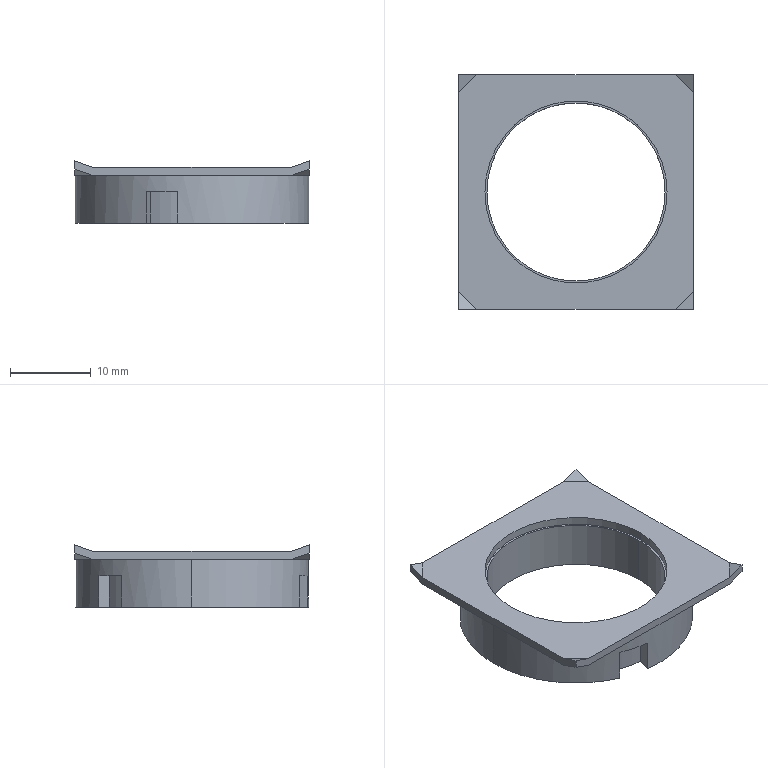Part | STEP file | A22NE_M_N_NUT | 1 solid | 34 faces | box 29 x 29 x 7.7 mm | volume 1960 mm3 | plane 25 | cylinder 9 | commonest cylinder face diameters 25.2 x3 22 x2 22.5 x2 28.8 x2
STEP:
#1=CARTESIAN_POINT('',(-11.25,0.,-0.8));
#2=VERTEX_POINT('',#1);
#3=CARTESIAN_POINT('',(11.25,0.,-0.8));
#4=VERTEX_POINT('',#3);
#5=CARTESIAN_POINT('',(0.,0.,-0.8));
#6=DIRECTION('',(0.,0.,1.));
#7=DIRECTION('',(1.,0.,0.));
#8=AXIS2_PLACEMENT_3D('',#5,#6,#7);
#9=CIRCLE('',#8,11.25);
#10=EDGE_CURVE('',#2,#4,#9,.T.);
#11=ORIENTED_EDGE('',*,*,#10,.T.);
#12=CARTESIAN_POINT('',(11.25,0.,-1.8));
#13=VERTEX_POINT('',#12);
#14=CARTESIAN_POINT('',(11.25,0.,-0.8));
#15=DIRECTION('',(0.,0.,-1.));
#16=VECTOR('',#15,1000.);
#17=LINE('',#14,#16);
#18=EDGE_CURVE('',#4,#13,#17,.T.);
#19=ORIENTED_EDGE('',*,*,#18,.T.);
#20=CARTESIAN_POINT('',(-11.25,0.,-1.8));
#21=VERTEX_POINT('',#20);
#22=CARTESIAN_POINT('',(0.,0.,-1.8));
#23=DIRECTION('',(0.,0.,-1.));
#24=DIRECTION('',(1.,0.,0.));
#25=AXIS2_PLACEMENT_3D('',#22,#23,#24);
#26=CIRCLE('',#25,11.25);
#27=EDGE_CURVE('',#13,#21,#26,.T.);
#28=ORIENTED_EDGE('',*,*,#27,.T.);
#29=CARTESIAN_POINT('',(-11.25,0.,-0.8));
#30=DIRECTION('',(0.,0.,-1.));
#31=VECTOR('',#30,1000.);
#32=LINE('',#29,#31);
#33=EDGE_CURVE('',#2,#21,#32,.T.);
#34=ORIENTED_EDGE('',*,*,#33,.F.);
#35=EDGE_LOOP('',(#11,#19,#28,#34));
#36=FACE_OUTER_BOUND('',#35,.T.);
#37=CARTESIAN_POINT('',(0.,0.,-0.8));
#38=DIRECTION('',(0.,0.,-1.));
#39=DIRECTION('',(-1.,0.,0.));
#40=AXIS2_PLACEMENT_3D('',#37,#38,#39);
#41=CYLINDRICAL_SURFACE('',#40,11.25);
#42=ADVANCED_FACE('',(#36),#41,.F.);
#43=CARTESIAN_POINT('',(-11.,0.,-7.7));
#44=VERTEX_POINT('',#43);
#45=CARTESIAN_POINT('',(11.,0.,-7.7));
#46=VERTEX_POINT('',#45);
#47=CARTESIAN_POINT('',(0.,0.,-7.7));
#48=DIRECTION('',(0.,0.,1.));
#49=DIRECTION('',(1.,0.,0.));
#50=AXIS2_PLACEMENT_3D('',#47,#48,#49);
#51=CIRCLE('',#50,11.);
#52=EDGE_CURVE('',#44,#46,#51,.T.);
#53=ORIENTED_EDGE('',*,*,#52,.F.);
#54=CARTESIAN_POINT('',(-11.,0.,-1.8));
#55=VERTEX_POINT('',#54);
#56=CARTESIAN_POINT('',(-11.,0.,-7.7));
#57=DIRECTION('',(0.,0.,1.));
#58=VECTOR('',#57,1000.);
#59=LINE('',#56,#58);
#60=EDGE_CURVE('',#44,#55,#59,.T.);
#61=ORIENTED_EDGE('',*,*,#60,.T.);
#62=CARTESIAN_POINT('',(11.,0.,-1.8));
#63=VERTEX_POINT('',#62);
#64=CARTESIAN_POINT('',(0.,0.,-1.8));
#65=DIRECTION('',(0.,0.,1.));
#66=DIRECTION('',(1.,0.,0.));
#67=AXIS2_PLACEMENT_3D('',#64,#65,#66);
#68=CIRCLE('',#67,11.);
#69=EDGE_CURVE('',#55,#63,#68,.T.);
#70=ORIENTED_EDGE('',*,*,#69,.T.);
#71=CARTESIAN_POINT('',(11.,0.,-7.7));
#72=DIRECTION('',(0.,0.,1.));
#73=VECTOR('',#72,1000.);
#74=LINE('',#71,#73);
#75=EDGE_CURVE('',#46,#63,#74,.T.);
#76=ORIENTED_EDGE('',*,*,#75,.F.);
#77=EDGE_LOOP('',(#53,#61,#70,#76));
#78=FACE_OUTER_BOUND('',#77,.T.);
#79=CARTESIAN_POINT('',(0.,0.,-7.7));
#80=DIRECTION('',(0.,0.,1.));
#81=DIRECTION('',(1.,0.,0.));
#82=AXIS2_PLACEMENT_3D('',#79,#80,#81);
#83=CYLINDRICAL_SURFACE('',#82,11.);
#84=ADVANCED_FACE('',(#78),#83,.F.);
#85=CARTESIAN_POINT('',(-11.498,8.669,-7.7));
#86=VERTEX_POINT('',#85);
#87=CARTESIAN_POINT('',(-14.4,0.,-7.7));
#88=VERTEX_POINT('',#87);
#89=CARTESIAN_POINT('',(0.,0.,-7.7));
#90=DIRECTION('',(0.,0.,1.));
#91=DIRECTION('',(1.,0.,0.));
#92=AXIS2_PLACEMENT_3D('',#89,#90,#91);
#93=CIRCLE('',#92,14.4);
#94=EDGE_CURVE('',#86,#88,#93,.T.);
#95=ORIENTED_EDGE('',*,*,#94,.T.);
#96=CARTESIAN_POINT('',(-14.4,0.,-1.8));
#97=VERTEX_POINT('',#96);
#98=CARTESIAN_POINT('',(-14.4,0.,-7.7));
#99=DIRECTION('',(0.,0.,1.));
#100=VECTOR('',#99,1000.);
#101=LINE('',#98,#100);
#102=EDGE_CURVE('',#88,#97,#101,.T.);
#103=ORIENTED_EDGE('',*,*,#102,.T.);
#104=CARTESIAN_POINT('',(14.4,0.,-1.8));
#105=VERTEX_POINT('',#104);
#106=CARTESIAN_POINT('',(0.,0.,-1.8));
#107=DIRECTION('',(0.,0.,1.));
#108=DIRECTION('',(1.,0.,0.));
#109=AXIS2_PLACEMENT_3D('',#106,#107,#108);
#110=CIRCLE('',#109,14.4);
#111=EDGE_CURVE('',#105,#97,#110,.T.);
#112=ORIENTED_EDGE('',*,*,#111,.F.);
#113=CARTESIAN_POINT('',(14.4,0.,-7.7));
#114=VERTEX_POINT('',#113);
#115=CARTESIAN_POINT('',(14.4,0.,-7.7));
#116=DIRECTION('',(0.,0.,1.));
#117=VECTOR('',#116,1000.);
#118=LINE('',#115,#117);
#119=EDGE_CURVE('',#114,#105,#118,.T.);
#120=ORIENTED_EDGE('',*,*,#119,.F.);
#121=CARTESIAN_POINT('',(14.292,1.759,-7.7));
#122=VERTEX_POINT('',#121);
#123=CARTESIAN_POINT('',(0.,0.,-7.7));
#124=DIRECTION('',(0.,0.,1.));
#125=DIRECTION('',(1.,0.,0.));
#126=AXIS2_PLACEMENT_3D('',#123,#124,#125);
#127=CIRCLE('',#126,14.4);
#128=EDGE_CURVE('',#114,#122,#127,.T.);
#129=ORIENTED_EDGE('',*,*,#128,.T.);
#130=CARTESIAN_POINT('',(14.292,1.759,-3.8));
#131=VERTEX_POINT('',#130);
#132=CARTESIAN_POINT('',(14.292,1.759,-3.8));
#133=DIRECTION('',(0.,0.,-1.));
#134=VECTOR('',#133,1000.);
#135=LINE('',#132,#134);
#136=EDGE_CURVE('',#131,#122,#135,.T.);
#137=ORIENTED_EDGE('',*,*,#136,.F.);
#138=CARTESIAN_POINT('',(13.257,5.623,-3.8));
#139=VERTEX_POINT('',#138);
#140=CARTESIAN_POINT('',(0.,0.,-3.8));
#141=DIRECTION('',(0.,0.,-1.));
#142=DIRECTION('',(0.5,0.866,0.));
#143=AXIS2_PLACEMENT_3D('',#140,#141,#142);
#144=CIRCLE('',#143,14.4);
#145=EDGE_CURVE('',#139,#131,#144,.T.);
#146=ORIENTED_EDGE('',*,*,#145,.F.);
#147=CARTESIAN_POINT('',(13.257,5.623,-7.7));
#148=VERTEX_POINT('',#147);
#149=CARTESIAN_POINT('',(13.257,5.623,-3.8));
#150=DIRECTION('',(0.,0.,-1.));
#151=VECTOR('',#150,1000.);
#152=LINE('',#149,#151);
#153=EDGE_CURVE('',#139,#148,#152,.T.);
#154=ORIENTED_EDGE('',*,*,#153,.T.);
#155=CARTESIAN_POINT('',(-8.669,11.498,-7.7));
#156=VERTEX_POINT('',#155);
#157=CARTESIAN_POINT('',(0.,0.,-7.7));
#158=DIRECTION('',(0.,0.,1.));
#159=DIRECTION('',(1.,0.,0.));
#160=AXIS2_PLACEMENT_3D('',#157,#158,#159);
#161=CIRCLE('',#160,14.4);
#162=EDGE_CURVE('',#148,#156,#161,.T.);
#163=ORIENTED_EDGE('',*,*,#162,.T.);
#164=CARTESIAN_POINT('',(-8.669,11.498,-3.8));
#165=VERTEX_POINT('',#164);
#166=CARTESIAN_POINT('',(-8.669,11.498,-3.8));
#167=DIRECTION('',(0.,0.,-1.));
#168=VECTOR('',#167,1000.);
#169=LINE('',#166,#168);
#170=EDGE_CURVE('',#165,#156,#169,.T.);
#171=ORIENTED_EDGE('',*,*,#170,.F.);
#172=CARTESIAN_POINT('',(-11.498,8.669,-3.8));
#173=VERTEX_POINT('',#172);
#174=CARTESIAN_POINT('',(0.,0.,-3.8));
#175=DIRECTION('',(0.,0.,-1.));
#176=DIRECTION('',(-1.,0.,0.));
#177=AXIS2_PLACEMENT_3D('',#174,#175,#176);
#178=CIRCLE('',#177,14.4);
#179=EDGE_CURVE('',#173,#165,#178,.T.);
#180=ORIENTED_EDGE('',*,*,#179,.F.);
#181=CARTESIAN_POINT('',(-11.498,8.669,-3.8));
#182=DIRECTION('',(0.,0.,-1.));
#183=VECTOR('',#182,1000.);
#184=LINE('',#181,#183);
#185=EDGE_CURVE('',#173,#86,#184,.T.);
#186=ORIENTED_EDGE('',*,*,#185,.T.);
#187=EDGE_LOOP('',(#95,#103,#112,#120,#129,#137,#146,#154,#163,#171,#180,#186));
#188=FACE_OUTER_BOUND('',#187,.T.);
#189=CARTESIAN_POINT('',(0.,0.,-7.7));
#190=DIRECTION('',(0.,0.,1.));
#191=DIRECTION('',(1.,0.,0.));
#192=AXIS2_PLACEMENT_3D('',#189,#190,#191);
#193=CYLINDRICAL_SURFACE('',#192,14.4);
#194=ADVANCED_FACE('',(#188),#193,.T.);
#195=ORIENTED_EDGE('',*,*,#102,.F.);
#196=CARTESIAN_POINT('',(-5.623,-13.257,-7.7));
#197=VERTEX_POINT('',#196);
#198=CARTESIAN_POINT('',(0.,0.,-7.7));
#199=DIRECTION('',(0.,0.,1.));
#200=DIRECTION('',(1.,0.,0.));
#201=AXIS2_PLACEMENT_3D('',#198,#199,#200);
#202=CIRCLE('',#201,14.4);
#203=EDGE_CURVE('',#88,#197,#202,.T.);
#204=ORIENTED_EDGE('',*,*,#203,.T.);
#205=CARTESIAN_POINT('',(-5.623,-13.257,-3.8));
#206=VERTEX_POINT('',#205);
#207=CARTESIAN_POINT('',(-5.623,-13.257,-3.8));
#208=DIRECTION('',(0.,0.,-1.));
#209=VECTOR('',#208,1000.);
#210=LINE('',#207,#209);
#211=EDGE_CURVE('',#206,#197,#210,.T.);
#212=ORIENTED_EDGE('',*,*,#211,.F.);
#213=CARTESIAN_POINT('',(-1.759,-14.292,-3.8));
#214=VERTEX_POINT('',#213);
#215=CARTESIAN_POINT('',(0.,0.,-3.8));
#216=DIRECTION('',(0.,0.,-1.));
#217=DIRECTION('',(0.5,-0.866,0.));
#218=AXIS2_PLACEMENT_3D('',#215,#216,#217);
#219=CIRCLE('',#218,14.4);
#220=EDGE_CURVE('',#214,#206,#219,.T.);
#221=ORIENTED_EDGE('',*,*,#220,.F.);
#222=CARTESIAN_POINT('',(-1.759,-14.292,-7.7));
#223=VERTEX_POINT('',#222);
#224=CARTESIAN_POINT('',(-1.759,-14.292,-3.8));
#225=DIRECTION('',(0.,0.,-1.));
#226=VECTOR('',#225,1000.);
#227=LINE('',#224,#226);
#228=EDGE_CURVE('',#214,#223,#227,.T.);
#229=ORIENTED_EDGE('',*,*,#228,.T.);
#230=CARTESIAN_POINT('',(0.,0.,-7.7));
#231=DIRECTION('',(0.,0.,1.));
#232=DIRECTION('',(1.,0.,0.));
#233=AXIS2_PLACEMENT_3D('',#230,#231,#232);
#234=CIRCLE('',#233,14.4);
#235=EDGE_CURVE('',#223,#114,#234,.T.);
#236=ORIENTED_EDGE('',*,*,#235,.T.);
#237=ORIENTED_EDGE('',*,*,#119,.T.);
#238=CARTESIAN_POINT('',(0.,0.,-1.8));
#239=DIRECTION('',(0.,0.,1.));
#240=DIRECTION('',(1.,0.,0.));
#241=AXIS2_PLACEMENT_3D('',#238,#239,#240);
#242=CIRCLE('',#241,14.4);
#243=EDGE_CURVE('',#97,#105,#242,.T.);
#244=ORIENTED_EDGE('',*,*,#243,.F.);
#245=EDGE_LOOP('',(#195,#204,#212,#221,#229,#236,#237,#244));
#246=FACE_OUTER_BOUND('',#245,.T.);
#247=CARTESIAN_POINT('',(0.,0.,-7.7));
#248=DIRECTION('',(0.,0.,1.));
#249=DIRECTION('',(1.,0.,0.));
#250=AXIS2_PLACEMENT_3D('',#247,#248,#249);
#251=CYLINDRICAL_SURFACE('',#250,14.4);
#252=ADVANCED_FACE('',(#246),#251,.T.);
#253=ORIENTED_EDGE('',*,*,#162,.F.);
#254=CARTESIAN_POINT('',(11.499,5.152,-7.7));
#255=VERTEX_POINT('',#254);
#256=CARTESIAN_POINT('',(13.257,5.623,-7.7));
#257=DIRECTION('',(0.9659,0.2588,0.));
#258=VECTOR('',#257,1000.);
#259=LINE('',#256,#258);
#260=EDGE_CURVE('',#255,#148,#259,.T.);
#261=ORIENTED_EDGE('',*,*,#260,.F.);
#262=CARTESIAN_POINT('',(12.534,1.288,-7.7));
#263=VERTEX_POINT('',#262);
#264=CARTESIAN_POINT('',(0.,0.,-7.7));
#265=DIRECTION('',(0.,0.,1.));
#266=DIRECTION('',(0.5,0.866,0.));
#267=AXIS2_PLACEMENT_3D('',#264,#265,#266);
#268=CIRCLE('',#267,12.6);
#269=EDGE_CURVE('',#263,#255,#268,.T.);
#270=ORIENTED_EDGE('',*,*,#269,.F.);
#271=CARTESIAN_POINT('',(14.292,1.759,-7.7));
#272=DIRECTION('',(-0.9659,-0.2588,0.));
#273=VECTOR('',#272,1000.);
#274=LINE('',#271,#273);
#275=EDGE_CURVE('',#122,#263,#274,.T.);
#276=ORIENTED_EDGE('',*,*,#275,.F.);
#277=ORIENTED_EDGE('',*,*,#128,.F.);
#278=ORIENTED_EDGE('',*,*,#235,.F.);
#279=CARTESIAN_POINT('',(-1.288,-12.534,-7.7));
#280=VERTEX_POINT('',#279);
#281=CARTESIAN_POINT('',(-1.759,-14.292,-7.7));
#282=DIRECTION('',(-0.2588,-0.9659,0.));
#283=VECTOR('',#282,1000.);
#284=LINE('',#281,#283);
#285=EDGE_CURVE('',#280,#223,#284,.T.);
#286=ORIENTED_EDGE('',*,*,#285,.F.);
#287=CARTESIAN_POINT('',(-5.152,-11.499,-7.7));
#288=VERTEX_POINT('',#287);
#289=CARTESIAN_POINT('',(0.,0.,-7.7));
#290=DIRECTION('',(0.,0.,1.));
#291=DIRECTION('',(0.5,-0.866,0.));
#292=AXIS2_PLACEMENT_3D('',#289,#290,#291);
#293=CIRCLE('',#292,12.6);
#294=EDGE_CURVE('',#288,#280,#293,.T.);
#295=ORIENTED_EDGE('',*,*,#294,.F.);
#296=CARTESIAN_POINT('',(-5.623,-13.257,-7.7));
#297=DIRECTION('',(0.2588,0.9659,0.));
#298=VECTOR('',#297,1000.);
#299=LINE('',#296,#298);
#300=EDGE_CURVE('',#197,#288,#299,.T.);
#301=ORIENTED_EDGE('',*,*,#300,.F.);
#302=ORIENTED_EDGE('',*,*,#203,.F.);
#303=ORIENTED_EDGE('',*,*,#94,.F.);
#304=CARTESIAN_POINT('',(-10.211,7.382,-7.7));
#305=VERTEX_POINT('',#304);
#306=CARTESIAN_POINT('',(-11.498,8.669,-7.7));
#307=DIRECTION('',(-0.7071,0.7071,0.));
#308=VECTOR('',#307,1000.);
#309=LINE('',#306,#308);
#310=EDGE_CURVE('',#305,#86,#309,.T.);
#311=ORIENTED_EDGE('',*,*,#310,.F.);
#312=CARTESIAN_POINT('',(-7.382,10.211,-7.7));
#313=VERTEX_POINT('',#312);
#314=CARTESIAN_POINT('',(0.,0.,-7.7));
#315=DIRECTION('',(0.,0.,1.));
#316=DIRECTION('',(-1.,0.,0.));
#317=AXIS2_PLACEMENT_3D('',#314,#315,#316);
#318=CIRCLE('',#317,12.6);
#319=EDGE_CURVE('',#313,#305,#318,.T.);
#320=ORIENTED_EDGE('',*,*,#319,.F.);
#321=CARTESIAN_POINT('',(-8.669,11.498,-7.7));
#322=DIRECTION('',(0.7071,-0.7071,0.));
#323=VECTOR('',#322,1000.);
#324=LINE('',#321,#323);
#325=EDGE_CURVE('',#156,#313,#324,.T.);
#326=ORIENTED_EDGE('',*,*,#325,.F.);
#327=EDGE_LOOP('',(#253,#261,#270,#276,#277,#278,#286,#295,#301,#302,#303,#311,#320,#326));
#328=FACE_OUTER_BOUND('',#327,.T.);
#329=CARTESIAN_POINT('',(0.,0.,-7.7));
#330=DIRECTION('',(0.,0.,1.));
#331=DIRECTION('',(1.,0.,0.));
#332=AXIS2_PLACEMENT_3D('',#329,#330,#331);
#333=CIRCLE('',#332,11.);
#334=EDGE_CURVE('',#46,#44,#333,.T.);
#335=ORIENTED_EDGE('',*,*,#334,.T.);
#336=ORIENTED_EDGE('',*,*,#52,.T.);
#337=EDGE_LOOP('',(#335,#336));
#338=FACE_BOUND('',#337,.T.);
#339=CARTESIAN_POINT('',(0.,0.,-7.7));
#340=DIRECTION('',(0.,0.,1.));
#341=DIRECTION('',(1.,0.,0.));
#342=AXIS2_PLACEMENT_3D('',#339,#340,#341);
#343=PLANE('',#342);
#344=ADVANCED_FACE('',(#328,#338),#343,.F.);
#345=CARTESIAN_POINT('',(0.,0.,-1.8));
#346=DIRECTION('',(0.,0.,-1.));
#347=DIRECTION('',(1.,0.,0.));
#348=AXIS2_PLACEMENT_3D('',#345,#346,#347);
#349=CIRCLE('',#348,11.25);
#350=EDGE_CURVE('',#21,#13,#349,.T.);
#351=ORIENTED_EDGE('',*,*,#350,.F.);
#352=ORIENTED_EDGE('',*,*,#27,.F.);
#353=EDGE_LOOP('',(#351,#352));
#354=FACE_OUTER_BOUND('',#353,.T.);
#355=CARTESIAN_POINT('',(0.,0.,-1.8));
#356=DIRECTION('',(0.,0.,1.));
#357=DIRECTION('',(1.,0.,0.));
#358=AXIS2_PLACEMENT_3D('',#355,#356,#357);
#359=CIRCLE('',#358,11.);
#360=EDGE_CURVE('',#63,#55,#359,.T.);
#361=ORIENTED_EDGE('',*,*,#360,.F.);
#362=ORIENTED_EDGE('',*,*,#69,.F.);
#363=EDGE_LOOP('',(#361,#362));
#364=FACE_BOUND('',#363,.T.);
#365=CARTESIAN_POINT('',(0.,0.,-1.8));
#366=DIRECTION('',(0.,0.,1.));
#367=DIRECTION('',(1.,0.,0.));
#368=AXIS2_PLACEMENT_3D('',#365,#366,#367);
#369=PLANE('',#368);
#370=ADVANCED_FACE('',(#354,#364),#369,.T.);
#371=ORIENTED_EDGE('',*,*,#60,.F.);
#372=ORIENTED_EDGE('',*,*,#334,.F.);
#373=ORIENTED_EDGE('',*,*,#75,.T.);
#374=ORIENTED_EDGE('',*,*,#360,.T.);
#375=EDGE_LOOP('',(#371,#372,#373,#374));
#376=FACE_OUTER_BOUND('',#375,.T.);
#377=CARTESIAN_POINT('',(0.,0.,-7.7));
#378=DIRECTION('',(0.,0.,1.));
#379=DIRECTION('',(1.,0.,0.));
#380=AXIS2_PLACEMENT_3D('',#377,#378,#379);
#381=CYLINDRICAL_SURFACE('',#380,11.);
#382=ADVANCED_FACE('',(#376),#381,.F.);
#383=ORIENTED_EDGE('',*,*,#310,.T.);
#384=ORIENTED_EDGE('',*,*,#185,.F.);
#385=CARTESIAN_POINT('',(-10.211,7.382,-3.8));
#386=VERTEX_POINT('',#385);
#387=CARTESIAN_POINT('',(-11.498,8.669,-3.8));
#388=DIRECTION('',(-0.7071,0.7071,0.));
#389=VECTOR('',#388,1000.);
#390=LINE('',#387,#389);
#391=EDGE_CURVE('',#386,#173,#390,.T.);
#392=ORIENTED_EDGE('',*,*,#391,.F.);
#393=CARTESIAN_POINT('',(-10.211,7.382,-3.8));
#394=DIRECTION('',(0.,0.,-1.));
#395=VECTOR('',#394,1000.);
#396=LINE('',#393,#395);
#397=EDGE_CURVE('',#386,#305,#396,.T.);
#398=ORIENTED_EDGE('',*,*,#397,.T.);
#399=EDGE_LOOP('',(#383,#384,#392,#398));
#400=FACE_OUTER_BOUND('',#399,.T.);
#401=CARTESIAN_POINT('',(-11.498,8.669,-3.8));
#402=DIRECTION('',(-0.7071,-0.7071,0.));
#403=DIRECTION('',(0.7071,-0.7071,0.));
#404=AXIS2_PLACEMENT_3D('',#401,#402,#403);
#405=PLANE('',#404);
#406=ADVANCED_FACE('',(#400),#405,.F.);
#407=ORIENTED_EDGE('',*,*,#319,.T.);
#408=ORIENTED_EDGE('',*,*,#397,.F.);
#409=CARTESIAN_POINT('',(-7.382,10.211,-3.8));
#410=VERTEX_POINT('',#409);
#411=CARTESIAN_POINT('',(0.,0.,-3.8));
#412=DIRECTION('',(0.,0.,1.));
#413=DIRECTION('',(-1.,0.,0.));
#414=AXIS2_PLACEMENT_3D('',#411,#412,#413);
#415=CIRCLE('',#414,12.6);
#416=EDGE_CURVE('',#410,#386,#415,.T.);
#417=ORIENTED_EDGE('',*,*,#416,.F.);
#418=CARTESIAN_POINT('',(-7.382,10.211,-3.8));
#419=DIRECTION('',(0.,0.,-1.));
#420=VECTOR('',#419,1000.);
#421=LINE('',#418,#420);
#422=EDGE_CURVE('',#410,#313,#421,.T.);
#423=ORIENTED_EDGE('',*,*,#422,.T.);
#424=EDGE_LOOP('',(#407,#408,#417,#423));
#425=FACE_OUTER_BOUND('',#424,.T.);
#426=CARTESIAN_POINT('',(0.,0.,-3.8));
#427=DIRECTION('',(0.,0.,-1.));
#428=DIRECTION('',(-1.,0.,0.));
#429=AXIS2_PLACEMENT_3D('',#426,#427,#428);
#430=CYLINDRICAL_SURFACE('',#429,12.6);
#431=ADVANCED_FACE('',(#425),#430,.T.);
#432=ORIENTED_EDGE('',*,*,#325,.T.);
#433=ORIENTED_EDGE('',*,*,#422,.F.);
#434=CARTESIAN_POINT('',(-8.669,11.498,-3.8));
#435=DIRECTION('',(0.7071,-0.7071,0.));
#436=VECTOR('',#435,1000.);
#437=LINE('',#434,#436);
#438=EDGE_CURVE('',#165,#410,#437,.T.);
#439=ORIENTED_EDGE('',*,*,#438,.F.);
#440=ORIENTED_EDGE('',*,*,#170,.T.);
#441=EDGE_LOOP('',(#432,#433,#439,#440));
#442=FACE_OUTER_BOUND('',#441,.T.);
#443=CARTESIAN_POINT('',(-8.669,11.498,-3.8));
#444=DIRECTION('',(0.7071,0.7071,0.));
#445=DIRECTION('',(-0.7071,0.7071,0.));
#446=AXIS2_PLACEMENT_3D('',#443,#444,#445);
#447=PLANE('',#446);
#448=ADVANCED_FACE('',(#442),#447,.F.);
#449=ORIENTED_EDGE('',*,*,#179,.T.);
#450=ORIENTED_EDGE('',*,*,#438,.T.);
#451=ORIENTED_EDGE('',*,*,#416,.T.);
#452=ORIENTED_EDGE('',*,*,#391,.T.);
#453=EDGE_LOOP('',(#449,#450,#451,#452));
#454=FACE_OUTER_BOUND('',#453,.T.);
#455=CARTESIAN_POINT('',(0.,0.,-3.8));
#456=DIRECTION('',(0.,0.,-1.));
#457=DIRECTION('',(-1.,0.,0.));
#458=AXIS2_PLACEMENT_3D('',#455,#456,#457);
#459=PLANE('',#458);
#460=ADVANCED_FACE('',(#454),#459,.T.);
#461=ORIENTED_EDGE('',*,*,#285,.T.);
#462=ORIENTED_EDGE('',*,*,#228,.F.);
#463=CARTESIAN_POINT('',(-1.288,-12.534,-3.8));
#464=VERTEX_POINT('',#463);
#465=CARTESIAN_POINT('',(-1.759,-14.292,-3.8));
#466=DIRECTION('',(-0.2588,-0.9659,0.));
#467=VECTOR('',#466,1000.);
#468=LINE('',#465,#467);
#469=EDGE_CURVE('',#464,#214,#468,.T.);
#470=ORIENTED_EDGE('',*,*,#469,.F.);
#471=CARTESIAN_POINT('',(-1.288,-12.534,-3.8));
#472=DIRECTION('',(0.,0.,-1.));
#473=VECTOR('',#472,1000.);
#474=LINE('',#471,#473);
#475=EDGE_CURVE('',#464,#280,#474,.T.);
#476=ORIENTED_EDGE('',*,*,#475,.T.);
#477=EDGE_LOOP('',(#461,#462,#470,#476));
#478=FACE_OUTER_BOUND('',#477,.T.);
#479=CARTESIAN_POINT('',(-1.759,-14.292,-3.8));
#480=DIRECTION('',(0.9659,-0.2588,0.));
#481=DIRECTION('',(0.2588,0.9659,0.));
#482=AXIS2_PLACEMENT_3D('',#479,#480,#481);
#483=PLANE('',#482);
#484=ADVANCED_FACE('',(#478),#483,.F.);
#485=ORIENTED_EDGE('',*,*,#294,.T.);
#486=ORIENTED_EDGE('',*,*,#475,.F.);
#487=CARTESIAN_POINT('',(-5.152,-11.499,-3.8));
#488=VERTEX_POINT('',#487);
#489=CARTESIAN_POINT('',(0.,0.,-3.8));
#490=DIRECTION('',(0.,0.,1.));
#491=DIRECTION('',(0.5,-0.866,0.));
#492=AXIS2_PLACEMENT_3D('',#489,#490,#491);
#493=CIRCLE('',#492,12.6);
#494=EDGE_CURVE('',#488,#464,#493,.T.);
#495=ORIENTED_EDGE('',*,*,#494,.F.);
#496=CARTESIAN_POINT('',(-5.152,-11.499,-3.8));
#497=DIRECTION('',(0.,0.,-1.));
#498=VECTOR('',#497,1000.);
#499=LINE('',#496,#498);
#500=EDGE_CURVE('',#488,#288,#499,.T.);
#501=ORIENTED_EDGE('',*,*,#500,.T.);
#502=EDGE_LOOP('',(#485,#486,#495,#501));
#503=FACE_OUTER_BOUND('',#502,.T.);
#504=CARTESIAN_POINT('',(0.,0.,-3.8));
#505=DIRECTION('',(0.,0.,-1.));
#506=DIRECTION('',(-1.,0.,0.));
#507=AXIS2_PLACEMENT_3D('',#504,#505,#506);
#508=CYLINDRICAL_SURFACE('',#507,12.6);
#509=ADVANCED_FACE('',(#503),#508,.T.);
#510=ORIENTED_EDGE('',*,*,#300,.T.);
#511=ORIENTED_EDGE('',*,*,#500,.F.);
#512=CARTESIAN_POINT('',(-5.623,-13.257,-3.8));
#513=DIRECTION('',(0.2588,0.9659,0.));
#514=VECTOR('',#513,1000.);
#515=LINE('',#512,#514);
#516=EDGE_CURVE('',#206,#488,#515,.T.);
#517=ORIENTED_EDGE('',*,*,#516,.F.);
#518=ORIENTED_EDGE('',*,*,#211,.T.);
#519=EDGE_LOOP('',(#510,#511,#517,#518));
#520=FACE_OUTER_BOUND('',#519,.T.);
#521=CARTESIAN_POINT('',(-5.623,-13.257,-3.8));
#522=DIRECTION('',(-0.9659,0.2588,0.));
#523=DIRECTION('',(-0.2588,-0.9659,0.));
#524=AXIS2_PLACEMENT_3D('',#521,#522,#523);
#525=PLANE('',#524);
#526=ADVANCED_FACE('',(#520),#525,.F.);
#527=ORIENTED_EDGE('',*,*,#220,.T.);
#528=ORIENTED_EDGE('',*,*,#516,.T.);
#529=ORIENTED_EDGE('',*,*,#494,.T.);
#530=ORIENTED_EDGE('',*,*,#469,.T.);
#531=EDGE_LOOP('',(#527,#528,#529,#530));
#532=FACE_OUTER_BOUND('',#531,.T.);
#533=CARTESIAN_POINT('',(0.,0.,-3.8));
#534=DIRECTION('',(0.,0.,-1.));
#535=DIRECTION('',(0.5,-0.866,0.));
#536=AXIS2_PLACEMENT_3D('',#533,#534,#535);
#537=PLANE('',#536);
#538=ADVANCED_FACE('',(#532),#537,.T.);
#539=ORIENTED_EDGE('',*,*,#260,.T.);
#540=ORIENTED_EDGE('',*,*,#153,.F.);
#541=CARTESIAN_POINT('',(11.499,5.152,-3.8));
#542=VERTEX_POINT('',#541);
#543=CARTESIAN_POINT('',(13.257,5.623,-3.8));
#544=DIRECTION('',(0.9659,0.2588,0.));
#545=VECTOR('',#544,1000.);
#546=LINE('',#543,#545);
#547=EDGE_CURVE('',#542,#139,#546,.T.);
#548=ORIENTED_EDGE('',*,*,#547,.F.);
#549=CARTESIAN_POINT('',(11.499,5.152,-3.8));
#550=DIRECTION('',(0.,0.,-1.));
#551=VECTOR('',#550,1000.);
#552=LINE('',#549,#551);
#553=EDGE_CURVE('',#542,#255,#552,.T.);
#554=ORIENTED_EDGE('',*,*,#553,.T.);
#555=EDGE_LOOP('',(#539,#540,#548,#554));
#556=FACE_OUTER_BOUND('',#555,.T.);
#557=CARTESIAN_POINT('',(13.257,5.623,-3.8));
#558=DIRECTION('',(-0.2588,0.9659,0.));
#559=DIRECTION('',(-0.9659,-0.2588,0.));
#560=AXIS2_PLACEMENT_3D('',#557,#558,#559);
#561=PLANE('',#560);
#562=ADVANCED_FACE('',(#556),#561,.F.);
#563=ORIENTED_EDGE('',*,*,#269,.T.);
#564=ORIENTED_EDGE('',*,*,#553,.F.);
#565=CARTESIAN_POINT('',(12.534,1.288,-3.8));
#566=VERTEX_POINT('',#565);
#567=CARTESIAN_POINT('',(0.,0.,-3.8));
#568=DIRECTION('',(0.,0.,1.));
#569=DIRECTION('',(0.5,0.866,0.));
#570=AXIS2_PLACEMENT_3D('',#567,#568,#569);
#571=CIRCLE('',#570,12.6);
#572=EDGE_CURVE('',#566,#542,#571,.T.);
#573=ORIENTED_EDGE('',*,*,#572,.F.);
#574=CARTESIAN_POINT('',(12.534,1.288,-3.8));
#575=DIRECTION('',(0.,0.,-1.));
#576=VECTOR('',#575,1000.);
#577=LINE('',#574,#576);
#578=EDGE_CURVE('',#566,#263,#577,.T.);
#579=ORIENTED_EDGE('',*,*,#578,.T.);
#580=EDGE_LOOP('',(#563,#564,#573,#579));
#581=FACE_OUTER_BOUND('',#580,.T.);
#582=CARTESIAN_POINT('',(0.,0.,-3.8));
#583=DIRECTION('',(0.,0.,-1.));
#584=DIRECTION('',(-1.,0.,0.));
#585=AXIS2_PLACEMENT_3D('',#582,#583,#584);
#586=CYLINDRICAL_SURFACE('',#585,12.6);
#587=ADVANCED_FACE('',(#581),#586,.T.);
#588=ORIENTED_EDGE('',*,*,#275,.T.);
#589=ORIENTED_EDGE('',*,*,#578,.F.);
#590=CARTESIAN_POINT('',(14.292,1.759,-3.8));
#591=DIRECTION('',(-0.9659,-0.2588,0.));
#592=VECTOR('',#591,1000.);
#593=LINE('',#590,#592);
#594=EDGE_CURVE('',#131,#566,#593,.T.);
#595=ORIENTED_EDGE('',*,*,#594,.F.);
#596=ORIENTED_EDGE('',*,*,#136,.T.);
#597=EDGE_LOOP('',(#588,#589,#595,#596));
#598=FACE_OUTER_BOUND('',#597,.T.);
#599=CARTESIAN_POINT('',(14.292,1.759,-3.8));
#600=DIRECTION('',(0.2588,-0.9659,0.));
#601=DIRECTION('',(0.9659,0.2588,0.));
#602=AXIS2_PLACEMENT_3D('',#599,#600,#601);
#603=PLANE('',#602);
#604=ADVANCED_FACE('',(#598),#603,.F.);
#605=ORIENTED_EDGE('',*,*,#145,.T.);
#606=ORIENTED_EDGE('',*,*,#594,.T.);
#607=ORIENTED_EDGE('',*,*,#572,.T.);
#608=ORIENTED_EDGE('',*,*,#547,.T.);
#609=EDGE_LOOP('',(#605,#606,#607,#608));
#610=FACE_OUTER_BOUND('',#609,.T.);
#611=CARTESIAN_POINT('',(0.,0.,-3.8));
#612=DIRECTION('',(0.,0.,-1.));
#613=DIRECTION('',(0.5,0.866,0.));
#614=AXIS2_PLACEMENT_3D('',#611,#612,#613);
#615=PLANE('',#614);
#616=ADVANCED_FACE('',(#610),#615,.T.);
#617=ORIENTED_EDGE('',*,*,#111,.T.);
#618=ORIENTED_EDGE('',*,*,#243,.T.);
#619=EDGE_LOOP('',(#617,#618));
#620=FACE_BOUND('',#619,.T.);
#621=CARTESIAN_POINT('',(14.5,12.25,-1.8));
#622=VERTEX_POINT('',#621);
#623=CARTESIAN_POINT('',(12.25,14.5,-1.8));
#624=VERTEX_POINT('',#623);
#625=CARTESIAN_POINT('',(12.25,14.5,-1.8));
#626=DIRECTION('',(-0.7071,0.7071,0.));
#627=VECTOR('',#626,1000.);
#628=LINE('',#625,#627);
#629=EDGE_CURVE('',#622,#624,#628,.T.);
#630=ORIENTED_EDGE('',*,*,#629,.F.);
#631=CARTESIAN_POINT('',(14.5,-12.25,-1.8));
#632=VERTEX_POINT('',#631);
#633=CARTESIAN_POINT('',(14.5,12.25,-1.8));
#634=DIRECTION('',(0.,1.,0.));
#635=VECTOR('',#634,1000.);
#636=LINE('',#633,#635);
#637=EDGE_CURVE('',#632,#622,#636,.T.);
#638=ORIENTED_EDGE('',*,*,#637,.F.);
#639=CARTESIAN_POINT('',(12.25,-14.5,-1.8));
#640=VERTEX_POINT('',#639);
#641=CARTESIAN_POINT('',(12.25,-14.5,-1.8));
#642=DIRECTION('',(0.7071,0.7071,0.));
#643=VECTOR('',#642,1000.);
#644=LINE('',#641,#643);
#645=EDGE_CURVE('',#640,#632,#644,.T.);
#646=ORIENTED_EDGE('',*,*,#645,.F.);
#647=CARTESIAN_POINT('',(-12.25,-14.5,-1.8));
#648=VERTEX_POINT('',#647);
#649=CARTESIAN_POINT('',(-12.25,-14.5,-1.8));
#650=DIRECTION('',(1.,0.,0.));
#651=VECTOR('',#650,1000.);
#652=LINE('',#649,#651);
#653=EDGE_CURVE('',#648,#640,#652,.T.);
#654=ORIENTED_EDGE('',*,*,#653,.F.);
#655=CARTESIAN_POINT('',(-14.5,-12.25,-1.8));
#656=VERTEX_POINT('',#655);
#657=CARTESIAN_POINT('',(-14.5,-12.25,-1.8));
#658=DIRECTION('',(0.7071,-0.7071,0.));
#659=VECTOR('',#658,1000.);
#660=LINE('',#657,#659);
#661=EDGE_CURVE('',#656,#648,#660,.T.);
#662=ORIENTED_EDGE('',*,*,#661,.F.);
#663=CARTESIAN_POINT('',(-14.5,12.25,-1.8));
#664=VERTEX_POINT('',#663);
#665=CARTESIAN_POINT('',(-14.5,12.25,-1.8));
#666=DIRECTION('',(0.,-1.,0.));
#667=VECTOR('',#666,1000.);
#668=LINE('',#665,#667);
#669=EDGE_CURVE('',#664,#656,#668,.T.);
#670=ORIENTED_EDGE('',*,*,#669,.F.);
#671=CARTESIAN_POINT('',(-12.25,14.5,-1.8));
#672=VERTEX_POINT('',#671);
#673=CARTESIAN_POINT('',(-14.5,12.25,-1.8));
#674=DIRECTION('',(-0.7071,-0.7071,0.));
#675=VECTOR('',#674,1000.);
#676=LINE('',#673,#675);
#677=EDGE_CURVE('',#672,#664,#676,.T.);
#678=ORIENTED_EDGE('',*,*,#677,.F.);
#679=CARTESIAN_POINT('',(-12.25,14.5,-1.8));
#680=DIRECTION('',(-1.,0.,0.));
#681=VECTOR('',#680,1000.);
#682=LINE('',#679,#681);
#683=EDGE_CURVE('',#624,#672,#682,.T.);
#684=ORIENTED_EDGE('',*,*,#683,.F.);
#685=EDGE_LOOP('',(#630,#638,#646,#654,#662,#670,#678,#684));
#686=FACE_OUTER_BOUND('',#685,.T.);
#687=CARTESIAN_POINT('',(26.75,0.,-1.8));
#688=DIRECTION('',(0.,0.,1.));
#689=DIRECTION('',(1.,0.,0.));
#690=AXIS2_PLACEMENT_3D('',#687,#688,#689);
#691=PLANE('',#690);
#692=ADVANCED_FACE('',(#620,#686),#691,.F.);
#693=CARTESIAN_POINT('',(14.5,12.25,-0.8));
#694=VERTEX_POINT('',#693);
#695=CARTESIAN_POINT('',(12.25,14.5,-0.8));
#696=VERTEX_POINT('',#695);
#697=CARTESIAN_POINT('',(12.25,14.5,-0.8));
#698=DIRECTION('',(-0.7071,0.7071,0.));
#699=VECTOR('',#698,1000.);
#700=LINE('',#697,#699);
#701=EDGE_CURVE('',#694,#696,#700,.T.);
#702=ORIENTED_EDGE('',*,*,#701,.T.);
#703=CARTESIAN_POINT('',(-12.25,14.5,-0.8));
#704=VERTEX_POINT('',#703);
#705=CARTESIAN_POINT('',(-12.25,14.5,-0.8));
#706=DIRECTION('',(-1.,0.,0.));
#707=VECTOR('',#706,1000.);
#708=LINE('',#705,#707);
#709=EDGE_CURVE('',#696,#704,#708,.T.);
#710=ORIENTED_EDGE('',*,*,#709,.T.);
#711=CARTESIAN_POINT('',(-14.5,12.25,-0.8));
#712=VERTEX_POINT('',#711);
#713=CARTESIAN_POINT('',(-14.5,12.25,-0.8));
#714=DIRECTION('',(-0.7071,-0.7071,0.));
#715=VECTOR('',#714,1000.);
#716=LINE('',#713,#715);
#717=EDGE_CURVE('',#704,#712,#716,.T.);
#718=ORIENTED_EDGE('',*,*,#717,.T.);
#719=CARTESIAN_POINT('',(-14.5,-12.25,-0.8));
#720=VERTEX_POINT('',#719);
#721=CARTESIAN_POINT('',(-14.5,12.25,-0.8));
#722=DIRECTION('',(0.,-1.,0.));
#723=VECTOR('',#722,1000.);
#724=LINE('',#721,#723);
#725=EDGE_CURVE('',#712,#720,#724,.T.);
#726=ORIENTED_EDGE('',*,*,#725,.T.);
#727=CARTESIAN_POINT('',(-12.25,-14.5,-0.8));
#728=VERTEX_POINT('',#727);
#729=CARTESIAN_POINT('',(-14.5,-12.25,-0.8));
#730=DIRECTION('',(0.7071,-0.7071,0.));
#731=VECTOR('',#730,1000.);
#732=LINE('',#729,#731);
#733=EDGE_CURVE('',#720,#728,#732,.T.);
#734=ORIENTED_EDGE('',*,*,#733,.T.);
#735=CARTESIAN_POINT('',(12.25,-14.5,-0.8));
#736=VERTEX_POINT('',#735);
#737=CARTESIAN_POINT('',(-12.25,-14.5,-0.8));
#738=DIRECTION('',(1.,0.,0.));
#739=VECTOR('',#738,1000.);
#740=LINE('',#737,#739);
#741=EDGE_CURVE('',#728,#736,#740,.T.);
#742=ORIENTED_EDGE('',*,*,#741,.T.);
#743=CARTESIAN_POINT('',(14.5,-12.25,-0.8));
#744=VERTEX_POINT('',#743);
#745=CARTESIAN_POINT('',(12.25,-14.5,-0.8));
#746=DIRECTION('',(0.7071,0.7071,0.));
#747=VECTOR('',#746,1000.);
#748=LINE('',#745,#747);
#749=EDGE_CURVE('',#736,#744,#748,.T.);
#750=ORIENTED_EDGE('',*,*,#749,.T.);
#751=CARTESIAN_POINT('',(14.5,12.25,-0.8));
#752=DIRECTION('',(0.,1.,0.));
#753=VECTOR('',#752,1000.);
#754=LINE('',#751,#753);
#755=EDGE_CURVE('',#744,#694,#754,.T.);
#756=ORIENTED_EDGE('',*,*,#755,.T.);
#757=EDGE_LOOP('',(#702,#710,#718,#726,#734,#742,#750,#756));
#758=FACE_OUTER_BOUND('',#757,.T.);
#759=ORIENTED_EDGE('',*,*,#10,.F.);
#760=CARTESIAN_POINT('',(0.,0.,-0.8));
#761=DIRECTION('',(0.,0.,1.));
#762=DIRECTION('',(1.,0.,0.));
#763=AXIS2_PLACEMENT_3D('',#760,#761,#762);
#764=CIRCLE('',#763,11.25);
#765=EDGE_CURVE('',#4,#2,#764,.T.);
#766=ORIENTED_EDGE('',*,*,#765,.F.);
#767=EDGE_LOOP('',(#759,#766));
#768=FACE_BOUND('',#767,.T.);
#769=CARTESIAN_POINT('',(26.75,0.,-0.8));
#770=DIRECTION('',(0.,0.,1.));
#771=DIRECTION('',(1.,0.,0.));
#772=AXIS2_PLACEMENT_3D('',#769,#770,#771);
#773=PLANE('',#772);
#774=ADVANCED_FACE('',(#758,#768),#773,.T.);
#775=ORIENTED_EDGE('',*,*,#683,.T.);
#776=CARTESIAN_POINT('',(-14.5,14.5,-1.));
#777=VERTEX_POINT('',#776);
#778=CARTESIAN_POINT('',(-12.18,14.5,-1.825));
#779=DIRECTION('',(0.9422,0.,-0.335));
#780=VECTOR('',#779,1000.);
#781=LINE('',#778,#780);
#782=EDGE_CURVE('',#777,#672,#781,.T.);
#783=ORIENTED_EDGE('',*,*,#782,.F.);
#784=CARTESIAN_POINT('',(-14.5,14.5,0.));
#785=VERTEX_POINT('',#784);
#786=CARTESIAN_POINT('',(-14.5,14.5,0.));
#787=DIRECTION('',(0.,0.,1.));
#788=VECTOR('',#787,1000.);
#789=LINE('',#786,#788);
#790=EDGE_CURVE('',#777,#785,#789,.T.);
#791=ORIENTED_EDGE('',*,*,#790,.T.);
#792=CARTESIAN_POINT('',(-10.929,14.5,-1.27));
#793=DIRECTION('',(-0.9422,0.,0.335));
#794=VECTOR('',#793,1000.);
#795=LINE('',#792,#794);
#796=EDGE_CURVE('',#704,#785,#795,.T.);
#797=ORIENTED_EDGE('',*,*,#796,.F.);
#798=ORIENTED_EDGE('',*,*,#709,.F.);
#799=CARTESIAN_POINT('',(14.5,14.5,0.));
#800=VERTEX_POINT('',#799);
#801=CARTESIAN_POINT('',(10.883,14.5,-1.286));
#802=DIRECTION('',(0.9422,0.,0.335));
#803=VECTOR('',#802,1000.);
#804=LINE('',#801,#803);
#805=EDGE_CURVE('',#696,#800,#804,.T.);
#806=ORIENTED_EDGE('',*,*,#805,.T.);
#807=CARTESIAN_POINT('',(14.5,14.5,-1.));
#808=VERTEX_POINT('',#807);
#809=CARTESIAN_POINT('',(14.5,14.5,0.));
#810=DIRECTION('',(0.,0.,-1.));
#811=VECTOR('',#810,1000.);
#812=LINE('',#809,#811);
#813=EDGE_CURVE('',#800,#808,#812,.T.);
#814=ORIENTED_EDGE('',*,*,#813,.T.);
#815=CARTESIAN_POINT('',(10.883,14.5,-2.286));
#816=DIRECTION('',(-0.9422,0.,-0.335));
#817=VECTOR('',#816,1000.);
#818=LINE('',#815,#817);
#819=EDGE_CURVE('',#808,#624,#818,.T.);
#820=ORIENTED_EDGE('',*,*,#819,.T.);
#821=EDGE_LOOP('',(#775,#783,#791,#797,#798,#806,#814,#820));
#822=FACE_OUTER_BOUND('',#821,.T.);
#823=CARTESIAN_POINT('',(-12.25,14.5,-0.8));
#824=DIRECTION('',(0.,-1.,0.));
#825=DIRECTION('',(1.,0.,0.));
#826=AXIS2_PLACEMENT_3D('',#823,#824,#825);
#827=PLANE('',#826);
#828=ADVANCED_FACE('',(#822),#827,.F.);
#829=ORIENTED_EDGE('',*,*,#669,.T.);
#830=CARTESIAN_POINT('',(-14.5,-14.5,-1.));
#831=VERTEX_POINT('',#830);
#832=CARTESIAN_POINT('',(-14.5,-10.883,-2.286));
#833=DIRECTION('',(0.,-0.9422,0.335));
#834=VECTOR('',#833,1000.);
#835=LINE('',#832,#834);
#836=EDGE_CURVE('',#656,#831,#835,.T.);
#837=ORIENTED_EDGE('',*,*,#836,.T.);
#838=CARTESIAN_POINT('',(-14.5,-14.5,0.));
#839=VERTEX_POINT('',#838);
#840=CARTESIAN_POINT('',(-14.5,-14.5,0.));
#841=DIRECTION('',(0.,0.,-1.));
#842=VECTOR('',#841,1000.);
#843=LINE('',#840,#842);
#844=EDGE_CURVE('',#839,#831,#843,.T.);
#845=ORIENTED_EDGE('',*,*,#844,.F.);
#846=CARTESIAN_POINT('',(-14.5,-12.134,-0.8412));
#847=DIRECTION('',(0.,0.9422,-0.335));
#848=VECTOR('',#847,1000.);
#849=LINE('',#846,#848);
#850=EDGE_CURVE('',#839,#720,#849,.T.);
#851=ORIENTED_EDGE('',*,*,#850,.T.);
#852=ORIENTED_EDGE('',*,*,#725,.F.);
#853=CARTESIAN_POINT('',(-14.5,10.929,-1.27));
#854=DIRECTION('',(0.,0.9422,0.335));
#855=VECTOR('',#854,1000.);
#856=LINE('',#853,#855);
#857=EDGE_CURVE('',#712,#785,#856,.T.);
#858=ORIENTED_EDGE('',*,*,#857,.T.);
#859=ORIENTED_EDGE('',*,*,#790,.F.);
#860=CARTESIAN_POINT('',(-14.5,12.18,-1.825));
#861=DIRECTION('',(0.,-0.9422,-0.335));
#862=VECTOR('',#861,1000.);
#863=LINE('',#860,#862);
#864=EDGE_CURVE('',#777,#664,#863,.T.);
#865=ORIENTED_EDGE('',*,*,#864,.T.);
#866=EDGE_LOOP('',(#829,#837,#845,#851,#852,#858,#859,#865));
#867=FACE_OUTER_BOUND('',#866,.T.);
#868=CARTESIAN_POINT('',(-14.5,12.25,-0.8));
#869=DIRECTION('',(1.,0.,0.));
#870=DIRECTION('',(0.,0.,-1.));
#871=AXIS2_PLACEMENT_3D('',#868,#869,#870);
#872=PLANE('',#871);
#873=ADVANCED_FACE('',(#867),#872,.F.);
#874=ORIENTED_EDGE('',*,*,#653,.T.);
#875=CARTESIAN_POINT('',(14.5,-14.5,-1.));
#876=VERTEX_POINT('',#875);
#877=CARTESIAN_POINT('',(12.18,-14.5,-1.825));
#878=DIRECTION('',(0.9422,0.,0.335));
#879=VECTOR('',#878,1000.);
#880=LINE('',#877,#879);
#881=EDGE_CURVE('',#640,#876,#880,.T.);
#882=ORIENTED_EDGE('',*,*,#881,.T.);
#883=CARTESIAN_POINT('',(14.5,-14.5,0.));
#884=VERTEX_POINT('',#883);
#885=CARTESIAN_POINT('',(14.5,-14.5,0.));
#886=DIRECTION('',(0.,0.,-1.));
#887=VECTOR('',#886,1000.);
#888=LINE('',#885,#887);
#889=EDGE_CURVE('',#884,#876,#888,.T.);
#890=ORIENTED_EDGE('',*,*,#889,.F.);
#891=CARTESIAN_POINT('',(10.929,-14.5,-1.27));
#892=DIRECTION('',(-0.9422,0.,-0.335));
#893=VECTOR('',#892,1000.);
#894=LINE('',#891,#893);
#895=EDGE_CURVE('',#884,#736,#894,.T.);
#896=ORIENTED_EDGE('',*,*,#895,.T.);
#897=ORIENTED_EDGE('',*,*,#741,.F.);
#898=CARTESIAN_POINT('',(-12.134,-14.5,-0.8412));
#899=DIRECTION('',(0.9422,0.,-0.335));
#900=VECTOR('',#899,1000.);
#901=LINE('',#898,#900);
#902=EDGE_CURVE('',#839,#728,#901,.T.);
#903=ORIENTED_EDGE('',*,*,#902,.F.);
#904=ORIENTED_EDGE('',*,*,#844,.T.);
#905=CARTESIAN_POINT('',(-10.883,-14.5,-2.286));
#906=DIRECTION('',(-0.9422,0.,0.335));
#907=VECTOR('',#906,1000.);
#908=LINE('',#905,#907);
#909=EDGE_CURVE('',#648,#831,#908,.T.);
#910=ORIENTED_EDGE('',*,*,#909,.F.);
#911=EDGE_LOOP('',(#874,#882,#890,#896,#897,#903,#904,#910));
#912=FACE_OUTER_BOUND('',#911,.T.);
#913=CARTESIAN_POINT('',(-12.25,-14.5,-0.8));
#914=DIRECTION('',(0.,1.,0.));
#915=DIRECTION('',(-1.,0.,0.));
#916=AXIS2_PLACEMENT_3D('',#913,#914,#915);
#917=PLANE('',#916);
#918=ADVANCED_FACE('',(#912),#917,.F.);
#919=ORIENTED_EDGE('',*,*,#637,.T.);
#920=CARTESIAN_POINT('',(14.5,10.883,-2.286));
#921=DIRECTION('',(0.,-0.9422,-0.335));
#922=VECTOR('',#921,1000.);
#923=LINE('',#920,#922);
#924=EDGE_CURVE('',#808,#622,#923,.T.);
#925=ORIENTED_EDGE('',*,*,#924,.F.);
#926=ORIENTED_EDGE('',*,*,#813,.F.);
#927=CARTESIAN_POINT('',(14.5,10.883,-1.286));
#928=DIRECTION('',(0.,0.9422,0.335));
#929=VECTOR('',#928,1000.);
#930=LINE('',#927,#929);
#931=EDGE_CURVE('',#694,#800,#930,.T.);
#932=ORIENTED_EDGE('',*,*,#931,.F.);
#933=ORIENTED_EDGE('',*,*,#755,.F.);
#934=CARTESIAN_POINT('',(14.5,-10.929,-1.27));
#935=DIRECTION('',(0.,0.9422,-0.335));
#936=VECTOR('',#935,1000.);
#937=LINE('',#934,#936);
#938=EDGE_CURVE('',#884,#744,#937,.T.);
#939=ORIENTED_EDGE('',*,*,#938,.F.);
#940=ORIENTED_EDGE('',*,*,#889,.T.);
#941=CARTESIAN_POINT('',(14.5,-12.18,-1.825));
#942=DIRECTION('',(0.,-0.9422,0.335));
#943=VECTOR('',#942,1000.);
#944=LINE('',#941,#943);
#945=EDGE_CURVE('',#632,#876,#944,.T.);
#946=ORIENTED_EDGE('',*,*,#945,.F.);
#947=EDGE_LOOP('',(#919,#925,#926,#932,#933,#939,#940,#946));
#948=FACE_OUTER_BOUND('',#947,.T.);
#949=CARTESIAN_POINT('',(14.5,12.25,-0.8));
#950=DIRECTION('',(-1.,0.,0.));
#951=DIRECTION('',(0.,-1.,0.));
#952=AXIS2_PLACEMENT_3D('',#949,#950,#951);
#953=PLANE('',#952);
#954=ADVANCED_FACE('',(#948),#953,.F.);
#955=ORIENTED_EDGE('',*,*,#18,.F.);
#956=ORIENTED_EDGE('',*,*,#765,.T.);
#957=ORIENTED_EDGE('',*,*,#33,.T.);
#958=ORIENTED_EDGE('',*,*,#350,.T.);
#959=EDGE_LOOP('',(#955,#956,#957,#958));
#960=FACE_OUTER_BOUND('',#959,.T.);
#961=CARTESIAN_POINT('',(0.,0.,-0.8));
#962=DIRECTION('',(0.,0.,-1.));
#963=DIRECTION('',(-1.,0.,0.));
#964=AXIS2_PLACEMENT_3D('',#961,#962,#963);
#965=CYLINDRICAL_SURFACE('',#964,11.25);
#966=ADVANCED_FACE('',(#960),#965,.F.);
#967=ORIENTED_EDGE('',*,*,#629,.T.);
#968=ORIENTED_EDGE('',*,*,#819,.F.);
#969=ORIENTED_EDGE('',*,*,#924,.T.);
#970=EDGE_LOOP('',(#967,#968,#969));
#971=FACE_OUTER_BOUND('',#970,.T.);
#972=CARTESIAN_POINT('',(16.04,10.71,-1.8));
#973=DIRECTION('',(-0.3177,-0.3177,0.8934));
#974=DIRECTION('',(0.,-0.9422,-0.335));
#975=AXIS2_PLACEMENT_3D('',#972,#973,#974);
#976=PLANE('',#975);
#977=ADVANCED_FACE('',(#971),#976,.F.);
#978=ORIENTED_EDGE('',*,*,#701,.F.);
#979=ORIENTED_EDGE('',*,*,#931,.T.);
#980=ORIENTED_EDGE('',*,*,#805,.F.);
#981=EDGE_LOOP('',(#978,#979,#980));
#982=FACE_OUTER_BOUND('',#981,.T.);
#983=CARTESIAN_POINT('',(16.04,10.71,-0.8));
#984=DIRECTION('',(0.3177,0.3177,-0.8934));
#985=DIRECTION('',(0.,0.9422,0.335));
#986=AXIS2_PLACEMENT_3D('',#983,#984,#985);
#987=PLANE('',#986);
#988=ADVANCED_FACE('',(#982),#987,.F.);
#989=ORIENTED_EDGE('',*,*,#733,.F.);
#990=ORIENTED_EDGE('',*,*,#850,.F.);
#991=ORIENTED_EDGE('',*,*,#902,.T.);
#992=EDGE_LOOP('',(#989,#990,#991));
#993=FACE_OUTER_BOUND('',#992,.T.);
#994=CARTESIAN_POINT('',(-11.835,-17.165,0.));
#995=DIRECTION('',(-0.3177,-0.3177,-0.8934));
#996=DIRECTION('',(0.,0.9422,-0.335));
#997=AXIS2_PLACEMENT_3D('',#994,#995,#996);
#998=PLANE('',#997);
#999=ADVANCED_FACE('',(#993),#998,.F.);
#1000=ORIENTED_EDGE('',*,*,#661,.T.);
#1001=ORIENTED_EDGE('',*,*,#909,.T.);
#1002=ORIENTED_EDGE('',*,*,#836,.F.);
#1003=EDGE_LOOP('',(#1000,#1001,#1002));
#1004=FACE_OUTER_BOUND('',#1003,.T.);
#1005=CARTESIAN_POINT('',(-10.71,-16.04,-1.8));
#1006=DIRECTION('',(0.3177,0.3177,0.8934));
#1007=DIRECTION('',(0.,-0.9422,0.335));
#1008=AXIS2_PLACEMENT_3D('',#1005,#1006,#1007);
#1009=PLANE('',#1008);
#1010=ADVANCED_FACE('',(#1004),#1009,.F.);
#1011=ORIENTED_EDGE('',*,*,#645,.T.);
#1012=ORIENTED_EDGE('',*,*,#945,.T.);
#1013=ORIENTED_EDGE('',*,*,#881,.F.);
#1014=EDGE_LOOP('',(#1011,#1012,#1013));
#1015=FACE_OUTER_BOUND('',#1014,.T.);
#1016=CARTESIAN_POINT('',(17.113,-11.887,-1.));
#1017=DIRECTION('',(-0.3177,0.3177,0.8934));
#1018=DIRECTION('',(0.9422,0.,0.335));
#1019=AXIS2_PLACEMENT_3D('',#1016,#1017,#1018);
#1020=PLANE('',#1019);
#1021=ADVANCED_FACE('',(#1015),#1020,.F.);
#1022=ORIENTED_EDGE('',*,*,#749,.F.);
#1023=ORIENTED_EDGE('',*,*,#895,.F.);
#1024=ORIENTED_EDGE('',*,*,#938,.T.);
#1025=EDGE_LOOP('',(#1022,#1023,#1024));
#1026=FACE_OUTER_BOUND('',#1025,.T.);
#1027=CARTESIAN_POINT('',(15.988,-10.762,-0.8));
#1028=DIRECTION('',(0.3177,-0.3177,-0.8934));
#1029=DIRECTION('',(-0.9422,0.,-0.335));
#1030=AXIS2_PLACEMENT_3D('',#1027,#1028,#1029);
#1031=PLANE('',#1030);
#1032=ADVANCED_FACE('',(#1026),#1031,.F.);
#1033=ORIENTED_EDGE('',*,*,#717,.F.);
#1034=ORIENTED_EDGE('',*,*,#796,.T.);
#1035=ORIENTED_EDGE('',*,*,#857,.F.);
#1036=EDGE_LOOP('',(#1033,#1034,#1035));
#1037=FACE_OUTER_BOUND('',#1036,.T.);
#1038=CARTESIAN_POINT('',(-10.762,15.988,-0.8));
#1039=DIRECTION('',(-0.3177,0.3177,-0.8934));
#1040=DIRECTION('',(-0.9422,0.,0.335));
#1041=AXIS2_PLACEMENT_3D('',#1038,#1039,#1040);
#1042=PLANE('',#1041);
#1043=ADVANCED_FACE('',(#1037),#1042,.F.);
#1044=ORIENTED_EDGE('',*,*,#677,.T.);
#1045=ORIENTED_EDGE('',*,*,#864,.F.);
#1046=ORIENTED_EDGE('',*,*,#782,.T.);
#1047=EDGE_LOOP('',(#1044,#1045,#1046));
#1048=FACE_OUTER_BOUND('',#1047,.T.);
#1049=CARTESIAN_POINT('',(-11.887,17.113,-1.));
#1050=DIRECTION('',(0.3177,-0.3177,0.8934));
#1051=DIRECTION('',(0.9422,0.,-0.335));
#1052=AXIS2_PLACEMENT_3D('',#1049,#1050,#1051);
#1053=PLANE('',#1052);
#1054=ADVANCED_FACE('',(#1048),#1053,.F.);
#1055=CLOSED_SHELL('',(#42,#84,#194,#252,#344,#370,#382,#406,#431,#448,#460,#484,#509,#526,#538,#562,#587,#604,#616,#692,#774,#828,#873,#918,#954,#966,#977,#988,#999,#1010,#1021,#1032,#1043,#1054));
#1056=MANIFOLD_SOLID_BREP('',#1055);
#1057=CARTESIAN_POINT('',(0.,0.,0.));
#1058=DIRECTION('',(0.,0.,1.));
#1059=DIRECTION('',(1.,0.,0.));
#1060=AXIS2_PLACEMENT_3D('',#1057,#1058,#1059);
#1061=(LENGTH_UNIT()NAMED_UNIT(*)SI_UNIT(.MILLI.,.METRE.));
#1062=UNCERTAINTY_MEASURE_WITH_UNIT(LENGTH_MEASURE(0.00001),#1061,'','');
#1063=(NAMED_UNIT(*)PLANE_ANGLE_UNIT()SI_UNIT($,.RADIAN.));
#1064=(NAMED_UNIT(*)SI_UNIT($,.STERADIAN.)SOLID_ANGLE_UNIT());
#1065=(GEOMETRIC_REPRESENTATION_CONTEXT(3)GLOBAL_UNCERTAINTY_ASSIGNED_CONTEXT((#1062))GLOBAL_UNIT_ASSIGNED_CONTEXT((#1061,#1063,#1064))REPRESENTATION_CONTEXT('',''));
#1066=ADVANCED_BREP_SHAPE_REPRESENTATION('',(#1056,#1060),#1065);